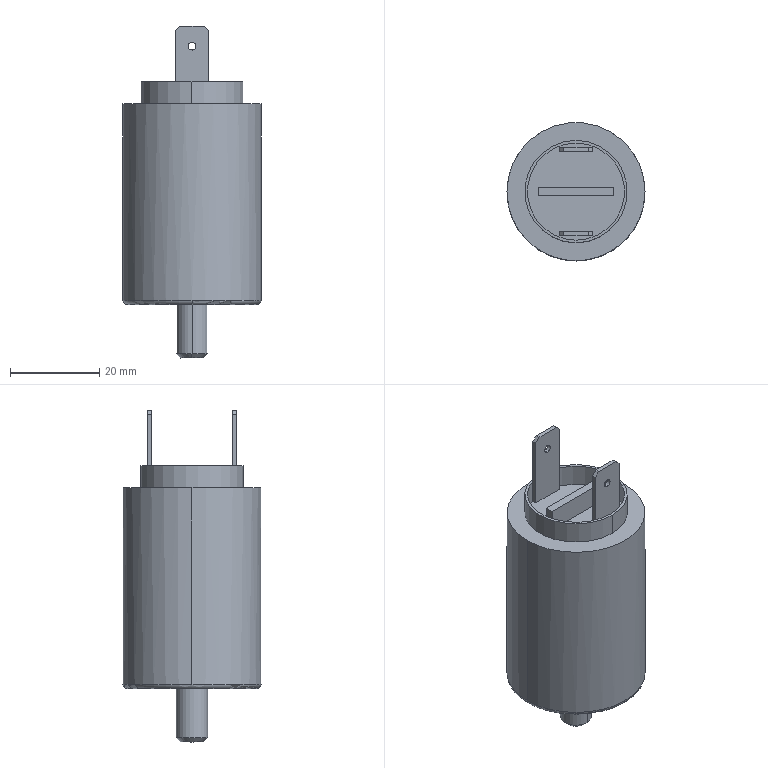Part | STEP file | MSBR-17_1_1_1_1 | 1 solid | 40 faces | box 31 x 31 x 74.5 mm | volume 34990 mm3 | plane 24 | cylinder 12 | torus 2 | cone 2 | commonest cylinder face diameters 1.8 x4 7 x2 21.8 x2 23 x2 31 x2
STEP:
#1=CARTESIAN_POINT('',(0.,0.,0.));
#2=DIRECTION('',(0.,0.,1.));
#3=DIRECTION('',(1.,0.,0.));
#4=AXIS2_PLACEMENT_3D('',#1,#2,#3);
#5=CARTESIAN_POINT('',(10.,61.412,67.3));
#6=VERTEX_POINT('',#5);
#7=CARTESIAN_POINT('',(10.,61.412,62.3));
#8=VERTEX_POINT('',#7);
#9=CARTESIAN_POINT('',(10.,61.412,67.3));
#10=DIRECTION('',(0.,0.,-1.));
#11=VECTOR('',#10,5.);
#12=LINE('',#9,#11);
#13=EDGE_CURVE('',#6,#8,#12,.T.);
#14=ORIENTED_EDGE('',*,*,#13,.F.);
#15=CARTESIAN_POINT('',(10.,83.212,67.3));
#16=VERTEX_POINT('',#15);
#17=CARTESIAN_POINT('',(10.,72.312,67.3));
#18=DIRECTION('',(0.,0.,1.));
#19=DIRECTION('',(0.,1.,0.));
#20=AXIS2_PLACEMENT_3D('',#17,#18,#19);
#21=CIRCLE('',#20,10.9);
#22=EDGE_CURVE('',#16,#6,#21,.T.);
#23=ORIENTED_EDGE('',*,*,#22,.F.);
#24=CARTESIAN_POINT('',(10.,83.212,62.3));
#25=VERTEX_POINT('',#24);
#26=CARTESIAN_POINT('',(10.,83.212,62.3));
#27=DIRECTION('',(0.,0.,1.));
#28=VECTOR('',#27,5.);
#29=LINE('',#26,#28);
#30=EDGE_CURVE('',#25,#16,#29,.T.);
#31=ORIENTED_EDGE('',*,*,#30,.F.);
#32=CARTESIAN_POINT('',(10.,72.312,62.3));
#33=DIRECTION('',(0.,0.,-1.));
#34=DIRECTION('',(0.,-1.,0.));
#35=AXIS2_PLACEMENT_3D('',#32,#33,#34);
#36=CIRCLE('',#35,10.9);
#37=EDGE_CURVE('',#8,#25,#36,.T.);
#38=ORIENTED_EDGE('',*,*,#37,.F.);
#39=EDGE_LOOP('',(#14,#23,#31,#38));
#40=FACE_OUTER_BOUND('',#39,.F.);
#41=CARTESIAN_POINT('',(10.,72.312,62.196));
#42=DIRECTION('',(0.,0.,1.));
#43=DIRECTION('',(0.,1.,0.));
#44=AXIS2_PLACEMENT_3D('',#41,#42,#43);
#45=CYLINDRICAL_SURFACE('',#44,10.9);
#46=ADVANCED_FACE('',(#40),#45,.F.);
#47=CARTESIAN_POINT('',(10.,72.312,67.3));
#48=DIRECTION('',(0.,0.,1.));
#49=DIRECTION('',(0.,-1.,0.));
#50=AXIS2_PLACEMENT_3D('',#47,#48,#49);
#51=CIRCLE('',#50,10.9);
#52=EDGE_CURVE('',#6,#16,#51,.T.);
#53=ORIENTED_EDGE('',*,*,#52,.F.);
#54=ORIENTED_EDGE('',*,*,#13,.T.);
#55=CARTESIAN_POINT('',(10.,72.312,62.3));
#56=DIRECTION('',(0.,0.,-1.));
#57=DIRECTION('',(0.,1.,0.));
#58=AXIS2_PLACEMENT_3D('',#55,#56,#57);
#59=CIRCLE('',#58,10.9);
#60=EDGE_CURVE('',#25,#8,#59,.T.);
#61=ORIENTED_EDGE('',*,*,#60,.F.);
#62=ORIENTED_EDGE('',*,*,#30,.T.);
#63=EDGE_LOOP('',(#53,#54,#61,#62));
#64=FACE_OUTER_BOUND('',#63,.F.);
#65=CARTESIAN_POINT('',(10.,72.312,62.196));
#66=DIRECTION('',(0.,0.,1.));
#67=DIRECTION('',(0.,-1.,0.));
#68=AXIS2_PLACEMENT_3D('',#65,#66,#67);
#69=CYLINDRICAL_SURFACE('',#68,10.9);
#70=ADVANCED_FACE('',(#64),#69,.F.);
#71=CARTESIAN_POINT('',(10.,83.812,67.3));
#72=VERTEX_POINT('',#71);
#73=CARTESIAN_POINT('',(10.,60.812,67.3));
#74=VERTEX_POINT('',#73);
#75=CARTESIAN_POINT('',(10.,72.312,67.3));
#76=DIRECTION('',(0.,0.,-1.));
#77=DIRECTION('',(0.,1.,0.));
#78=AXIS2_PLACEMENT_3D('',#75,#76,#77);
#79=CIRCLE('',#78,11.5);
#80=EDGE_CURVE('',#72,#74,#79,.T.);
#81=ORIENTED_EDGE('',*,*,#80,.T.);
#82=CARTESIAN_POINT('',(10.,72.312,67.3));
#83=DIRECTION('',(0.,0.,-1.));
#84=DIRECTION('',(0.,-1.,0.));
#85=AXIS2_PLACEMENT_3D('',#82,#83,#84);
#86=CIRCLE('',#85,11.5);
#87=EDGE_CURVE('',#74,#72,#86,.T.);
#88=ORIENTED_EDGE('',*,*,#87,.T.);
#89=EDGE_LOOP('',(#81,#88));
#90=FACE_OUTER_BOUND('',#89,.F.);
#91=ORIENTED_EDGE('',*,*,#22,.T.);
#92=ORIENTED_EDGE('',*,*,#52,.T.);
#93=EDGE_LOOP('',(#91,#92));
#94=FACE_BOUND('',#93,.F.);
#95=CARTESIAN_POINT('',(10.,72.312,67.3));
#96=DIRECTION('',(0.,0.,1.));
#97=DIRECTION('',(0.,1.,0.));
#98=AXIS2_PLACEMENT_3D('',#95,#96,#97);
#99=PLANE('',#98);
#100=ADVANCED_FACE('',(#90,#94),#99,.T.);
#101=CARTESIAN_POINT('',(10.,60.812,62.3));
#102=VERTEX_POINT('',#101);
#103=CARTESIAN_POINT('',(10.,83.812,62.3));
#104=VERTEX_POINT('',#103);
#105=CARTESIAN_POINT('',(10.,72.312,62.3));
#106=DIRECTION('',(0.,0.,1.));
#107=DIRECTION('',(0.,-1.,0.));
#108=AXIS2_PLACEMENT_3D('',#105,#106,#107);
#109=CIRCLE('',#108,11.5);
#110=EDGE_CURVE('',#102,#104,#109,.T.);
#111=ORIENTED_EDGE('',*,*,#110,.F.);
#112=CARTESIAN_POINT('',(10.,60.812,67.3));
#113=DIRECTION('',(0.,0.,-1.));
#114=VECTOR('',#113,5.);
#115=LINE('',#112,#114);
#116=EDGE_CURVE('',#74,#102,#115,.T.);
#117=ORIENTED_EDGE('',*,*,#116,.F.);
#118=ORIENTED_EDGE('',*,*,#80,.F.);
#119=CARTESIAN_POINT('',(10.,83.812,62.3));
#120=DIRECTION('',(0.,0.,1.));
#121=VECTOR('',#120,5.);
#122=LINE('',#119,#121);
#123=EDGE_CURVE('',#104,#72,#122,.T.);
#124=ORIENTED_EDGE('',*,*,#123,.F.);
#125=EDGE_LOOP('',(#111,#117,#118,#124));
#126=FACE_OUTER_BOUND('',#125,.F.);
#127=CARTESIAN_POINT('',(10.,72.312,62.196));
#128=DIRECTION('',(0.,0.,1.));
#129=DIRECTION('',(0.,-1.,0.));
#130=AXIS2_PLACEMENT_3D('',#127,#128,#129);
#131=CYLINDRICAL_SURFACE('',#130,11.5);
#132=ADVANCED_FACE('',(#126),#131,.T.);
#133=CARTESIAN_POINT('',(25.5,72.312,62.3));
#134=VERTEX_POINT('',#133);
#135=CARTESIAN_POINT('',(-5.5,72.312,62.3));
#136=VERTEX_POINT('',#135);
#137=CARTESIAN_POINT('',(10.,72.312,62.3));
#138=DIRECTION('',(0.,0.,-1.));
#139=DIRECTION('',(1.,0.,0.));
#140=AXIS2_PLACEMENT_3D('',#137,#138,#139);
#141=CIRCLE('',#140,15.5);
#142=EDGE_CURVE('',#134,#136,#141,.T.);
#143=ORIENTED_EDGE('',*,*,#142,.T.);
#144=CARTESIAN_POINT('',(10.,72.312,62.3));
#145=DIRECTION('',(0.,0.,-1.));
#146=DIRECTION('',(-1.,0.,0.));
#147=AXIS2_PLACEMENT_3D('',#144,#145,#146);
#148=CIRCLE('',#147,15.5);
#149=EDGE_CURVE('',#136,#134,#148,.T.);
#150=ORIENTED_EDGE('',*,*,#149,.T.);
#151=EDGE_LOOP('',(#143,#150));
#152=FACE_OUTER_BOUND('',#151,.F.);
#153=ORIENTED_EDGE('',*,*,#110,.T.);
#154=CARTESIAN_POINT('',(10.,72.312,62.3));
#155=DIRECTION('',(0.,0.,1.));
#156=DIRECTION('',(0.,1.,0.));
#157=AXIS2_PLACEMENT_3D('',#154,#155,#156);
#158=CIRCLE('',#157,11.5);
#159=EDGE_CURVE('',#104,#102,#158,.T.);
#160=ORIENTED_EDGE('',*,*,#159,.T.);
#161=EDGE_LOOP('',(#153,#160));
#162=FACE_BOUND('',#161,.F.);
#163=CARTESIAN_POINT('',(10.,72.312,62.3));
#164=DIRECTION('',(0.,0.,1.));
#165=DIRECTION('',(0.,1.,0.));
#166=AXIS2_PLACEMENT_3D('',#163,#164,#165);
#167=PLANE('',#166);
#168=ADVANCED_FACE('',(#152,#162),#167,.T.);
#169=CARTESIAN_POINT('',(10.,56.812,18.3));
#170=VERTEX_POINT('',#169);
#171=CARTESIAN_POINT('',(25.5,72.312,18.3));
#172=VERTEX_POINT('',#171);
#173=CARTESIAN_POINT('',(10.,72.312,18.3));
#174=DIRECTION('',(0.,0.,1.));
#175=DIRECTION('',(0.,-1.,0.));
#176=AXIS2_PLACEMENT_3D('',#173,#174,#175);
#177=CIRCLE('',#176,15.5);
#178=EDGE_CURVE('',#170,#172,#177,.T.);
#179=ORIENTED_EDGE('',*,*,#178,.F.);
#180=CARTESIAN_POINT('',(-5.5,72.312,18.3));
#181=VERTEX_POINT('',#180);
#182=CARTESIAN_POINT('',(10.,72.312,18.3));
#183=DIRECTION('',(0.,0.,1.));
#184=DIRECTION('',(-1.,0.,0.));
#185=AXIS2_PLACEMENT_3D('',#182,#183,#184);
#186=CIRCLE('',#185,15.5);
#187=EDGE_CURVE('',#181,#170,#186,.T.);
#188=ORIENTED_EDGE('',*,*,#187,.F.);
#189=CARTESIAN_POINT('',(-5.5,72.312,62.3));
#190=DIRECTION('',(0.,0.,-1.));
#191=VECTOR('',#190,44.);
#192=LINE('',#189,#191);
#193=EDGE_CURVE('',#136,#181,#192,.T.);
#194=ORIENTED_EDGE('',*,*,#193,.F.);
#195=ORIENTED_EDGE('',*,*,#142,.F.);
#196=CARTESIAN_POINT('',(25.5,72.312,18.3));
#197=DIRECTION('',(0.,0.,1.));
#198=VECTOR('',#197,44.);
#199=LINE('',#196,#198);
#200=EDGE_CURVE('',#172,#134,#199,.T.);
#201=ORIENTED_EDGE('',*,*,#200,.F.);
#202=EDGE_LOOP('',(#179,#188,#194,#195,#201));
#203=FACE_OUTER_BOUND('',#202,.F.);
#204=CARTESIAN_POINT('',(10.,72.312,17.42));
#205=DIRECTION('',(0.,0.,1.));
#206=DIRECTION('',(-1.,0.,0.));
#207=AXIS2_PLACEMENT_3D('',#204,#205,#206);
#208=CYLINDRICAL_SURFACE('',#207,15.5);
#209=ADVANCED_FACE('',(#203),#208,.T.);
#210=CARTESIAN_POINT('',(10.,57.812,17.3));
#211=VERTEX_POINT('',#210);
#212=CARTESIAN_POINT('',(10.,86.812,17.3));
#213=VERTEX_POINT('',#212);
#214=CARTESIAN_POINT('',(10.,72.312,17.3));
#215=DIRECTION('',(0.,0.,1.));
#216=DIRECTION('',(0.,-1.,0.));
#217=AXIS2_PLACEMENT_3D('',#214,#215,#216);
#218=CIRCLE('',#217,14.5);
#219=EDGE_CURVE('',#211,#213,#218,.T.);
#220=ORIENTED_EDGE('',*,*,#219,.F.);
#221=CARTESIAN_POINT('',(10.,57.812,18.3));
#222=DIRECTION('',(1.,0.,0.));
#223=DIRECTION('',(0.,-1.,0.));
#224=AXIS2_PLACEMENT_3D('',#221,#222,#223);
#225=CIRCLE('',#224,1.);
#226=EDGE_CURVE('',#170,#211,#225,.T.);
#227=ORIENTED_EDGE('',*,*,#226,.F.);
#228=ORIENTED_EDGE('',*,*,#178,.T.);
#229=CARTESIAN_POINT('',(10.,87.812,18.3));
#230=VERTEX_POINT('',#229);
#231=CARTESIAN_POINT('',(10.,72.312,18.3));
#232=DIRECTION('',(0.,0.,1.));
#233=DIRECTION('',(1.,0.,0.));
#234=AXIS2_PLACEMENT_3D('',#231,#232,#233);
#235=CIRCLE('',#234,15.5);
#236=EDGE_CURVE('',#172,#230,#235,.T.);
#237=ORIENTED_EDGE('',*,*,#236,.T.);
#238=CARTESIAN_POINT('',(10.,86.812,18.3));
#239=DIRECTION('',(1.,0.,0.));
#240=DIRECTION('',(0.,0.,-1.));
#241=AXIS2_PLACEMENT_3D('',#238,#239,#240);
#242=CIRCLE('',#241,1.);
#243=EDGE_CURVE('',#213,#230,#242,.T.);
#244=ORIENTED_EDGE('',*,*,#243,.F.);
#245=EDGE_LOOP('',(#220,#227,#228,#237,#244));
#246=FACE_OUTER_BOUND('',#245,.F.);
#247=CARTESIAN_POINT('',(10.,72.312,18.3));
#248=DIRECTION('',(0.,0.,-1.));
#249=DIRECTION('',(0.,-1.,0.));
#250=AXIS2_PLACEMENT_3D('',#247,#248,#249);
#251=TOROIDAL_SURFACE('',#250,14.5,1.);
#252=ADVANCED_FACE('',(#246),#251,.T.);
#253=ORIENTED_EDGE('',*,*,#219,.T.);
#254=CARTESIAN_POINT('',(10.,72.312,17.3));
#255=DIRECTION('',(0.,0.,1.));
#256=DIRECTION('',(0.,1.,0.));
#257=AXIS2_PLACEMENT_3D('',#254,#255,#256);
#258=CIRCLE('',#257,14.5);
#259=EDGE_CURVE('',#213,#211,#258,.T.);
#260=ORIENTED_EDGE('',*,*,#259,.T.);
#261=EDGE_LOOP('',(#253,#260));
#262=FACE_OUTER_BOUND('',#261,.F.);
#263=CARTESIAN_POINT('',(10.,75.812,17.3));
#264=VERTEX_POINT('',#263);
#265=CARTESIAN_POINT('',(10.,68.812,17.3));
#266=VERTEX_POINT('',#265);
#267=CARTESIAN_POINT('',(10.,72.312,17.3));
#268=DIRECTION('',(0.,0.,-1.));
#269=DIRECTION('',(0.,1.,0.));
#270=AXIS2_PLACEMENT_3D('',#267,#268,#269);
#271=CIRCLE('',#270,3.5);
#272=EDGE_CURVE('',#264,#266,#271,.T.);
#273=ORIENTED_EDGE('',*,*,#272,.T.);
#274=CARTESIAN_POINT('',(10.,72.312,17.3));
#275=DIRECTION('',(0.,0.,-1.));
#276=DIRECTION('',(0.,-1.,0.));
#277=AXIS2_PLACEMENT_3D('',#274,#275,#276);
#278=CIRCLE('',#277,3.5);
#279=EDGE_CURVE('',#266,#264,#278,.T.);
#280=ORIENTED_EDGE('',*,*,#279,.T.);
#281=EDGE_LOOP('',(#273,#280));
#282=FACE_BOUND('',#281,.F.);
#283=CARTESIAN_POINT('',(10.,72.312,17.3));
#284=DIRECTION('',(0.,0.,1.));
#285=DIRECTION('',(0.,1.,0.));
#286=AXIS2_PLACEMENT_3D('',#283,#284,#285);
#287=PLANE('',#286);
#288=ADVANCED_FACE('',(#262,#282),#287,.F.);
#289=ORIENTED_EDGE('',*,*,#243,.T.);
#290=CARTESIAN_POINT('',(10.,72.312,18.3));
#291=DIRECTION('',(0.,0.,1.));
#292=DIRECTION('',(0.,1.,0.));
#293=AXIS2_PLACEMENT_3D('',#290,#291,#292);
#294=CIRCLE('',#293,15.5);
#295=EDGE_CURVE('',#230,#181,#294,.T.);
#296=ORIENTED_EDGE('',*,*,#295,.T.);
#297=ORIENTED_EDGE('',*,*,#187,.T.);
#298=ORIENTED_EDGE('',*,*,#226,.T.);
#299=ORIENTED_EDGE('',*,*,#259,.F.);
#300=EDGE_LOOP('',(#289,#296,#297,#298,#299));
#301=FACE_OUTER_BOUND('',#300,.F.);
#302=CARTESIAN_POINT('',(10.,72.312,18.3));
#303=DIRECTION('',(0.,0.,-1.));
#304=DIRECTION('',(0.,1.,0.));
#305=AXIS2_PLACEMENT_3D('',#302,#303,#304);
#306=TOROIDAL_SURFACE('',#305,14.5,1.);
#307=ADVANCED_FACE('',(#301),#306,.T.);
#308=ORIENTED_EDGE('',*,*,#200,.T.);
#309=ORIENTED_EDGE('',*,*,#149,.F.);
#310=ORIENTED_EDGE('',*,*,#193,.T.);
#311=ORIENTED_EDGE('',*,*,#295,.F.);
#312=ORIENTED_EDGE('',*,*,#236,.F.);
#313=EDGE_LOOP('',(#308,#309,#310,#311,#312));
#314=FACE_OUTER_BOUND('',#313,.F.);
#315=CARTESIAN_POINT('',(10.,72.312,17.42));
#316=DIRECTION('',(0.,0.,1.));
#317=DIRECTION('',(1.,0.,0.));
#318=AXIS2_PLACEMENT_3D('',#315,#316,#317);
#319=CYLINDRICAL_SURFACE('',#318,15.5);
#320=ADVANCED_FACE('',(#314),#319,.T.);
#321=CARTESIAN_POINT('',(10.,68.812,6.3));
#322=VERTEX_POINT('',#321);
#323=CARTESIAN_POINT('',(10.,75.812,6.3));
#324=VERTEX_POINT('',#323);
#325=CARTESIAN_POINT('',(10.,72.312,6.3));
#326=DIRECTION('',(0.,0.,1.));
#327=DIRECTION('',(0.,-1.,0.));
#328=AXIS2_PLACEMENT_3D('',#325,#326,#327);
#329=CIRCLE('',#328,3.5);
#330=EDGE_CURVE('',#322,#324,#329,.T.);
#331=ORIENTED_EDGE('',*,*,#330,.F.);
#332=CARTESIAN_POINT('',(10.,68.812,17.3));
#333=DIRECTION('',(0.,-0.000000002,-1.));
#334=VECTOR('',#333,11.);
#335=LINE('',#332,#334);
#336=EDGE_CURVE('',#266,#322,#335,.T.);
#337=ORIENTED_EDGE('',*,*,#336,.F.);
#338=ORIENTED_EDGE('',*,*,#272,.F.);
#339=CARTESIAN_POINT('',(10.,75.812,6.3));
#340=DIRECTION('',(0.,-0.000000002,1.));
#341=VECTOR('',#340,11.);
#342=LINE('',#339,#341);
#343=EDGE_CURVE('',#324,#264,#342,.T.);
#344=ORIENTED_EDGE('',*,*,#343,.F.);
#345=EDGE_LOOP('',(#331,#337,#338,#344));
#346=FACE_OUTER_BOUND('',#345,.F.);
#347=CARTESIAN_POINT('',(10.,72.312,6.08));
#348=DIRECTION('',(0.,0.,1.));
#349=DIRECTION('',(0.,-1.,0.));
#350=AXIS2_PLACEMENT_3D('',#347,#348,#349);
#351=CYLINDRICAL_SURFACE('',#350,3.5);
#352=ADVANCED_FACE('',(#346),#351,.T.);
#353=ORIENTED_EDGE('',*,*,#330,.T.);
#354=CARTESIAN_POINT('',(10.,74.812,5.3));
#355=VERTEX_POINT('',#354);
#356=CARTESIAN_POINT('',(10.,74.812,5.3));
#357=DIRECTION('',(-0.000000004,0.7071,0.7071));
#358=VECTOR('',#357,1.414);
#359=LINE('',#356,#358);
#360=EDGE_CURVE('',#355,#324,#359,.T.);
#361=ORIENTED_EDGE('',*,*,#360,.F.);
#362=CARTESIAN_POINT('',(10.,69.812,5.3));
#363=VERTEX_POINT('',#362);
#364=CARTESIAN_POINT('',(10.,72.312,5.3));
#365=DIRECTION('',(0.,0.,1.));
#366=DIRECTION('',(0.,-1.,0.));
#367=AXIS2_PLACEMENT_3D('',#364,#365,#366);
#368=CIRCLE('',#367,2.5);
#369=EDGE_CURVE('',#363,#355,#368,.T.);
#370=ORIENTED_EDGE('',*,*,#369,.F.);
#371=CARTESIAN_POINT('',(10.,68.812,6.3));
#372=DIRECTION('',(0.,0.7071,-0.7071));
#373=VECTOR('',#372,1.414);
#374=LINE('',#371,#373);
#375=EDGE_CURVE('',#322,#363,#374,.T.);
#376=ORIENTED_EDGE('',*,*,#375,.F.);
#377=EDGE_LOOP('',(#353,#361,#370,#376));
#378=FACE_OUTER_BOUND('',#377,.F.);
#379=CARTESIAN_POINT('',(10.,72.312,5.8));
#380=DIRECTION('',(0.,0.,1.));
#381=DIRECTION('',(0.,1.,0.));
#382=AXIS2_PLACEMENT_3D('',#379,#380,#381);
#383=CONICAL_SURFACE('',#382,3.,45.);
#384=ADVANCED_FACE('',(#378),#383,.T.);
#385=ORIENTED_EDGE('',*,*,#375,.T.);
#386=CARTESIAN_POINT('',(10.,72.312,5.3));
#387=DIRECTION('',(-0.000000001,0.,1.));
#388=DIRECTION('',(0.000000006,1.,0.));
#389=AXIS2_PLACEMENT_3D('',#386,#387,#388);
#390=CIRCLE('',#389,2.5);
#391=EDGE_CURVE('',#355,#363,#390,.T.);
#392=ORIENTED_EDGE('',*,*,#391,.F.);
#393=ORIENTED_EDGE('',*,*,#360,.T.);
#394=CARTESIAN_POINT('',(10.,72.312,6.3));
#395=DIRECTION('',(-0.000000001,0.,1.));
#396=DIRECTION('',(0.,1.,0.));
#397=AXIS2_PLACEMENT_3D('',#394,#395,#396);
#398=CIRCLE('',#397,3.5);
#399=EDGE_CURVE('',#324,#322,#398,.T.);
#400=ORIENTED_EDGE('',*,*,#399,.T.);
#401=EDGE_LOOP('',(#385,#392,#393,#400));
#402=FACE_OUTER_BOUND('',#401,.F.);
#403=CARTESIAN_POINT('',(10.,72.312,5.8));
#404=DIRECTION('',(-0.000000001,0.,1.));
#405=DIRECTION('',(0.,-1.,0.));
#406=AXIS2_PLACEMENT_3D('',#403,#404,#405);
#407=CONICAL_SURFACE('',#406,3.,45.);
#408=ADVANCED_FACE('',(#402),#407,.T.);
#409=ORIENTED_EDGE('',*,*,#391,.T.);
#410=ORIENTED_EDGE('',*,*,#369,.T.);
#411=EDGE_LOOP('',(#409,#410));
#412=FACE_OUTER_BOUND('',#411,.F.);
#413=CARTESIAN_POINT('',(10.,72.312,5.3));
#414=DIRECTION('',(0.,0.,1.));
#415=DIRECTION('',(0.,1.,0.));
#416=AXIS2_PLACEMENT_3D('',#413,#414,#415);
#417=PLANE('',#416);
#418=ADVANCED_FACE('',(#412),#417,.F.);
#419=ORIENTED_EDGE('',*,*,#343,.T.);
#420=ORIENTED_EDGE('',*,*,#279,.F.);
#421=ORIENTED_EDGE('',*,*,#336,.T.);
#422=ORIENTED_EDGE('',*,*,#399,.F.);
#423=EDGE_LOOP('',(#419,#420,#421,#422));
#424=FACE_OUTER_BOUND('',#423,.F.);
#425=CARTESIAN_POINT('',(10.,72.312,6.08));
#426=DIRECTION('',(0.,0.,1.));
#427=DIRECTION('',(0.,1.,0.));
#428=AXIS2_PLACEMENT_3D('',#425,#426,#427);
#429=CYLINDRICAL_SURFACE('',#428,3.5);
#430=ADVANCED_FACE('',(#424),#429,.T.);
#431=ORIENTED_EDGE('',*,*,#123,.T.);
#432=ORIENTED_EDGE('',*,*,#87,.F.);
#433=ORIENTED_EDGE('',*,*,#116,.T.);
#434=ORIENTED_EDGE('',*,*,#159,.F.);
#435=EDGE_LOOP('',(#431,#432,#433,#434));
#436=FACE_OUTER_BOUND('',#435,.F.);
#437=CARTESIAN_POINT('',(10.,72.312,62.196));
#438=DIRECTION('',(0.,0.,1.));
#439=DIRECTION('',(0.,1.,0.));
#440=AXIS2_PLACEMENT_3D('',#437,#438,#439);
#441=CYLINDRICAL_SURFACE('',#440,11.5);
#442=ADVANCED_FACE('',(#436),#441,.T.);
#443=ORIENTED_EDGE('',*,*,#60,.T.);
#444=ORIENTED_EDGE('',*,*,#37,.T.);
#445=EDGE_LOOP('',(#443,#444));
#446=FACE_OUTER_BOUND('',#445,.F.);
#447=CARTESIAN_POINT('',(1.5,71.412,62.3));
#448=VERTEX_POINT('',#447);
#449=CARTESIAN_POINT('',(1.5,73.212,62.3));
#450=VERTEX_POINT('',#449);
#451=CARTESIAN_POINT('',(1.5,71.412,62.3));
#452=DIRECTION('',(0.,1.,0.));
#453=VECTOR('',#452,1.8);
#454=LINE('',#451,#453);
#455=EDGE_CURVE('',#448,#450,#454,.T.);
#456=ORIENTED_EDGE('',*,*,#455,.F.);
#457=CARTESIAN_POINT('',(18.5,71.412,62.3));
#458=VERTEX_POINT('',#457);
#459=CARTESIAN_POINT('',(18.5,71.412,62.3));
#460=DIRECTION('',(-1.,0.,0.));
#461=VECTOR('',#460,17.);
#462=LINE('',#459,#461);
#463=EDGE_CURVE('',#458,#448,#462,.T.);
#464=ORIENTED_EDGE('',*,*,#463,.F.);
#465=CARTESIAN_POINT('',(18.5,73.212,62.3));
#466=VERTEX_POINT('',#465);
#467=CARTESIAN_POINT('',(18.5,73.212,62.3));
#468=DIRECTION('',(0.,-1.,0.));
#469=VECTOR('',#468,1.8);
#470=LINE('',#467,#469);
#471=EDGE_CURVE('',#466,#458,#470,.T.);
#472=ORIENTED_EDGE('',*,*,#471,.F.);
#473=CARTESIAN_POINT('',(1.5,73.212,62.3));
#474=DIRECTION('',(1.,0.,0.));
#475=VECTOR('',#474,17.);
#476=LINE('',#473,#475);
#477=EDGE_CURVE('',#450,#466,#476,.T.);
#478=ORIENTED_EDGE('',*,*,#477,.F.);
#479=EDGE_LOOP('',(#456,#464,#472,#478));
#480=FACE_BOUND('',#479,.F.);
#481=CARTESIAN_POINT('',(13.75,82.212,62.3));
#482=VERTEX_POINT('',#481);
#483=CARTESIAN_POINT('',(13.75,81.312,62.3));
#484=VERTEX_POINT('',#483);
#485=CARTESIAN_POINT('',(13.75,82.212,62.3));
#486=DIRECTION('',(0.,-1.,0.));
#487=VECTOR('',#486,0.9);
#488=LINE('',#485,#487);
#489=EDGE_CURVE('',#482,#484,#488,.T.);
#490=ORIENTED_EDGE('',*,*,#489,.F.);
#491=CARTESIAN_POINT('',(6.25,82.212,62.3));
#492=VERTEX_POINT('',#491);
#493=CARTESIAN_POINT('',(6.25,82.212,62.3));
#494=DIRECTION('',(1.,0.,0.));
#495=VECTOR('',#494,7.5);
#496=LINE('',#493,#495);
#497=EDGE_CURVE('',#492,#482,#496,.T.);
#498=ORIENTED_EDGE('',*,*,#497,.F.);
#499=CARTESIAN_POINT('',(6.25,81.312,62.3));
#500=VERTEX_POINT('',#499);
#501=CARTESIAN_POINT('',(6.25,81.312,62.3));
#502=DIRECTION('',(0.,1.,0.));
#503=VECTOR('',#502,0.9);
#504=LINE('',#501,#503);
#505=EDGE_CURVE('',#500,#492,#504,.T.);
#506=ORIENTED_EDGE('',*,*,#505,.F.);
#507=CARTESIAN_POINT('',(13.75,81.312,62.3));
#508=DIRECTION('',(-1.,0.,0.));
#509=VECTOR('',#508,7.5);
#510=LINE('',#507,#509);
#511=EDGE_CURVE('',#484,#500,#510,.T.);
#512=ORIENTED_EDGE('',*,*,#511,.F.);
#513=EDGE_LOOP('',(#490,#498,#506,#512));
#514=FACE_BOUND('',#513,.F.);
#515=CARTESIAN_POINT('',(13.75,63.312,62.3));
#516=VERTEX_POINT('',#515);
#517=CARTESIAN_POINT('',(13.75,62.412,62.3));
#518=VERTEX_POINT('',#517);
#519=CARTESIAN_POINT('',(13.75,63.312,62.3));
#520=DIRECTION('',(0.,-1.,0.));
#521=VECTOR('',#520,0.9);
#522=LINE('',#519,#521);
#523=EDGE_CURVE('',#516,#518,#522,.T.);
#524=ORIENTED_EDGE('',*,*,#523,.F.);
#525=CARTESIAN_POINT('',(6.25,63.312,62.3));
#526=VERTEX_POINT('',#525);
#527=CARTESIAN_POINT('',(6.25,63.312,62.3));
#528=DIRECTION('',(1.,0.,0.));
#529=VECTOR('',#528,7.5);
#530=LINE('',#527,#529);
#531=EDGE_CURVE('',#526,#516,#530,.T.);
#532=ORIENTED_EDGE('',*,*,#531,.F.);
#533=CARTESIAN_POINT('',(6.25,62.412,62.3));
#534=VERTEX_POINT('',#533);
#535=CARTESIAN_POINT('',(6.25,62.412,62.3));
#536=DIRECTION('',(0.,1.,0.));
#537=VECTOR('',#536,0.9);
#538=LINE('',#535,#537);
#539=EDGE_CURVE('',#534,#526,#538,.T.);
#540=ORIENTED_EDGE('',*,*,#539,.F.);
#541=CARTESIAN_POINT('',(13.75,62.412,62.3));
#542=DIRECTION('',(-1.,0.,0.));
#543=VECTOR('',#542,7.5);
#544=LINE('',#541,#543);
#545=EDGE_CURVE('',#518,#534,#544,.T.);
#546=ORIENTED_EDGE('',*,*,#545,.F.);
#547=EDGE_LOOP('',(#524,#532,#540,#546));
#548=FACE_BOUND('',#547,.F.);
#549=CARTESIAN_POINT('',(10.,72.312,62.3));
#550=DIRECTION('',(0.,0.,1.));
#551=DIRECTION('',(0.,1.,0.));
#552=AXIS2_PLACEMENT_3D('',#549,#550,#551);
#553=PLANE('',#552);
#554=ADVANCED_FACE('',(#446,#480,#514,#548),#553,.T.);
#555=ORIENTED_EDGE('',*,*,#455,.T.);
#556=CARTESIAN_POINT('',(1.5,73.212,67.3));
#557=VERTEX_POINT('',#556);
#558=CARTESIAN_POINT('',(1.5,73.212,67.3));
#559=DIRECTION('',(0.,0.,-1.));
#560=VECTOR('',#559,5.);
#561=LINE('',#558,#560);
#562=EDGE_CURVE('',#557,#450,#561,.T.);
#563=ORIENTED_EDGE('',*,*,#562,.F.);
#564=CARTESIAN_POINT('',(1.5,71.412,67.3));
#565=VERTEX_POINT('',#564);
#566=CARTESIAN_POINT('',(1.5,71.412,67.3));
#567=DIRECTION('',(0.,1.,0.));
#568=VECTOR('',#567,1.8);
#569=LINE('',#566,#568);
#570=EDGE_CURVE('',#565,#557,#569,.T.);
#571=ORIENTED_EDGE('',*,*,#570,.F.);
#572=CARTESIAN_POINT('',(1.5,71.412,62.3));
#573=DIRECTION('',(0.,0.,1.));
#574=VECTOR('',#573,5.);
#575=LINE('',#572,#574);
#576=EDGE_CURVE('',#448,#565,#575,.T.);
#577=ORIENTED_EDGE('',*,*,#576,.F.);
#578=EDGE_LOOP('',(#555,#563,#571,#577));
#579=FACE_OUTER_BOUND('',#578,.F.);
#580=CARTESIAN_POINT('',(1.5,72.312,64.8));
#581=DIRECTION('',(1.,0.,0.));
#582=DIRECTION('',(0.,1.,0.));
#583=AXIS2_PLACEMENT_3D('',#580,#581,#582);
#584=PLANE('',#583);
#585=ADVANCED_FACE('',(#579),#584,.F.);
#586=ORIENTED_EDGE('',*,*,#477,.T.);
#587=CARTESIAN_POINT('',(18.5,73.212,67.3));
#588=VERTEX_POINT('',#587);
#589=CARTESIAN_POINT('',(18.5,73.212,67.3));
#590=DIRECTION('',(0.,0.,-1.));
#591=VECTOR('',#590,5.);
#592=LINE('',#589,#591);
#593=EDGE_CURVE('',#588,#466,#592,.T.);
#594=ORIENTED_EDGE('',*,*,#593,.F.);
#595=CARTESIAN_POINT('',(1.5,73.212,67.3));
#596=DIRECTION('',(1.,0.,0.));
#597=VECTOR('',#596,17.);
#598=LINE('',#595,#597);
#599=EDGE_CURVE('',#557,#588,#598,.T.);
#600=ORIENTED_EDGE('',*,*,#599,.F.);
#601=ORIENTED_EDGE('',*,*,#562,.T.);
#602=EDGE_LOOP('',(#586,#594,#600,#601));
#603=FACE_OUTER_BOUND('',#602,.F.);
#604=CARTESIAN_POINT('',(10.,73.212,64.8));
#605=DIRECTION('',(0.,1.,0.));
#606=DIRECTION('',(1.,0.,0.));
#607=AXIS2_PLACEMENT_3D('',#604,#605,#606);
#608=PLANE('',#607);
#609=ADVANCED_FACE('',(#603),#608,.T.);
#610=ORIENTED_EDGE('',*,*,#471,.T.);
#611=CARTESIAN_POINT('',(18.5,71.412,67.3));
#612=VERTEX_POINT('',#611);
#613=CARTESIAN_POINT('',(18.5,71.412,67.3));
#614=DIRECTION('',(0.,0.,-1.));
#615=VECTOR('',#614,5.);
#616=LINE('',#613,#615);
#617=EDGE_CURVE('',#612,#458,#616,.T.);
#618=ORIENTED_EDGE('',*,*,#617,.F.);
#619=CARTESIAN_POINT('',(18.5,73.212,67.3));
#620=DIRECTION('',(0.,-1.,0.));
#621=VECTOR('',#620,1.8);
#622=LINE('',#619,#621);
#623=EDGE_CURVE('',#588,#612,#622,.T.);
#624=ORIENTED_EDGE('',*,*,#623,.F.);
#625=ORIENTED_EDGE('',*,*,#593,.T.);
#626=EDGE_LOOP('',(#610,#618,#624,#625));
#627=FACE_OUTER_BOUND('',#626,.F.);
#628=CARTESIAN_POINT('',(18.5,72.312,64.8));
#629=DIRECTION('',(1.,0.,0.));
#630=DIRECTION('',(0.,-1.,0.));
#631=AXIS2_PLACEMENT_3D('',#628,#629,#630);
#632=PLANE('',#631);
#633=ADVANCED_FACE('',(#627),#632,.T.);
#634=ORIENTED_EDGE('',*,*,#463,.T.);
#635=ORIENTED_EDGE('',*,*,#576,.T.);
#636=CARTESIAN_POINT('',(18.5,71.412,67.3));
#637=DIRECTION('',(-1.,0.,0.));
#638=VECTOR('',#637,17.);
#639=LINE('',#636,#638);
#640=EDGE_CURVE('',#612,#565,#639,.T.);
#641=ORIENTED_EDGE('',*,*,#640,.F.);
#642=ORIENTED_EDGE('',*,*,#617,.T.);
#643=EDGE_LOOP('',(#634,#635,#641,#642));
#644=FACE_OUTER_BOUND('',#643,.F.);
#645=CARTESIAN_POINT('',(10.,71.412,64.8));
#646=DIRECTION('',(0.,1.,0.));
#647=DIRECTION('',(-1.,0.,0.));
#648=AXIS2_PLACEMENT_3D('',#645,#646,#647);
#649=PLANE('',#648);
#650=ADVANCED_FACE('',(#644),#649,.F.);
#651=ORIENTED_EDGE('',*,*,#570,.T.);
#652=ORIENTED_EDGE('',*,*,#599,.T.);
#653=ORIENTED_EDGE('',*,*,#623,.T.);
#654=ORIENTED_EDGE('',*,*,#640,.T.);
#655=EDGE_LOOP('',(#651,#652,#653,#654));
#656=FACE_OUTER_BOUND('',#655,.F.);
#657=CARTESIAN_POINT('',(10.,72.312,67.3));
#658=DIRECTION('',(0.,0.,1.));
#659=DIRECTION('',(0.,1.,0.));
#660=AXIS2_PLACEMENT_3D('',#657,#658,#659);
#661=PLANE('',#660);
#662=ADVANCED_FACE('',(#656),#661,.T.);
#663=CARTESIAN_POINT('',(13.75,82.212,78.8));
#664=VERTEX_POINT('',#663);
#665=CARTESIAN_POINT('',(13.75,82.212,62.3));
#666=DIRECTION('',(0.,0.,1.));
#667=VECTOR('',#666,16.5);
#668=LINE('',#665,#667);
#669=EDGE_CURVE('',#482,#664,#668,.T.);
#670=ORIENTED_EDGE('',*,*,#669,.F.);
#671=ORIENTED_EDGE('',*,*,#489,.T.);
#672=CARTESIAN_POINT('',(13.75,81.312,78.8));
#673=VERTEX_POINT('',#672);
#674=CARTESIAN_POINT('',(13.75,81.312,78.8));
#675=DIRECTION('',(0.,0.,-1.));
#676=VECTOR('',#675,16.5);
#677=LINE('',#674,#676);
#678=EDGE_CURVE('',#673,#484,#677,.T.);
#679=ORIENTED_EDGE('',*,*,#678,.F.);
#680=CARTESIAN_POINT('',(13.75,82.212,78.8));
#681=DIRECTION('',(0.,-1.,0.));
#682=VECTOR('',#681,0.9);
#683=LINE('',#680,#682);
#684=EDGE_CURVE('',#664,#673,#683,.T.);
#685=ORIENTED_EDGE('',*,*,#684,.F.);
#686=EDGE_LOOP('',(#670,#671,#679,#685));
#687=FACE_OUTER_BOUND('',#686,.F.);
#688=CARTESIAN_POINT('',(13.75,81.762,70.55));
#689=DIRECTION('',(1.,0.,0.));
#690=DIRECTION('',(0.,1.,0.));
#691=AXIS2_PLACEMENT_3D('',#688,#689,#690);
#692=PLANE('',#691);
#693=ADVANCED_FACE('',(#687),#692,.T.);
#694=CARTESIAN_POINT('',(6.25,82.212,78.8));
#695=VERTEX_POINT('',#694);
#696=CARTESIAN_POINT('',(6.25,82.212,62.3));
#697=DIRECTION('',(0.,0.,1.));
#698=VECTOR('',#697,16.5);
#699=LINE('',#696,#698);
#700=EDGE_CURVE('',#492,#695,#699,.T.);
#701=ORIENTED_EDGE('',*,*,#700,.F.);
#702=ORIENTED_EDGE('',*,*,#497,.T.);
#703=ORIENTED_EDGE('',*,*,#669,.T.);
#704=CARTESIAN_POINT('',(12.75,82.212,79.8));
#705=VERTEX_POINT('',#704);
#706=CARTESIAN_POINT('',(13.75,82.212,78.8));
#707=DIRECTION('',(-0.7071,0.,0.7071));
#708=VECTOR('',#707,1.414);
#709=LINE('',#706,#708);
#710=EDGE_CURVE('',#664,#705,#709,.T.);
#711=ORIENTED_EDGE('',*,*,#710,.T.);
#712=CARTESIAN_POINT('',(7.25,82.212,79.8));
#713=VERTEX_POINT('',#712);
#714=CARTESIAN_POINT('',(7.25,82.212,79.8));
#715=DIRECTION('',(1.,0.,0.));
#716=VECTOR('',#715,5.5);
#717=LINE('',#714,#716);
#718=EDGE_CURVE('',#713,#705,#717,.T.);
#719=ORIENTED_EDGE('',*,*,#718,.F.);
#720=CARTESIAN_POINT('',(7.25,82.212,79.8));
#721=DIRECTION('',(-0.7071,0.,-0.7071));
#722=VECTOR('',#721,1.414);
#723=LINE('',#720,#722);
#724=EDGE_CURVE('',#713,#695,#723,.T.);
#725=ORIENTED_EDGE('',*,*,#724,.T.);
#726=EDGE_LOOP('',(#701,#702,#703,#711,#719,#725));
#727=FACE_OUTER_BOUND('',#726,.F.);
#728=CARTESIAN_POINT('',(10.,82.212,74.4));
#729=VERTEX_POINT('',#728);
#730=CARTESIAN_POINT('',(10.,82.212,76.2));
#731=VERTEX_POINT('',#730);
#732=CARTESIAN_POINT('',(10.,82.212,75.3));
#733=DIRECTION('',(0.,1.,0.));
#734=DIRECTION('',(0.,0.,-1.));
#735=AXIS2_PLACEMENT_3D('',#732,#733,#734);
#736=CIRCLE('',#735,0.9);
#737=EDGE_CURVE('',#729,#731,#736,.T.);
#738=ORIENTED_EDGE('',*,*,#737,.T.);
#739=CARTESIAN_POINT('',(10.,82.212,75.3));
#740=DIRECTION('',(0.,1.,0.));
#741=DIRECTION('',(0.,0.,1.));
#742=AXIS2_PLACEMENT_3D('',#739,#740,#741);
#743=CIRCLE('',#742,0.9);
#744=EDGE_CURVE('',#731,#729,#743,.T.);
#745=ORIENTED_EDGE('',*,*,#744,.T.);
#746=EDGE_LOOP('',(#738,#745));
#747=FACE_BOUND('',#746,.F.);
#748=CARTESIAN_POINT('',(10.,82.212,71.05));
#749=DIRECTION('',(0.,1.,0.));
#750=DIRECTION('',(-1.,0.,0.));
#751=AXIS2_PLACEMENT_3D('',#748,#749,#750);
#752=PLANE('',#751);
#753=ADVANCED_FACE('',(#727,#747),#752,.T.);
#754=CARTESIAN_POINT('',(6.25,81.312,78.8));
#755=VERTEX_POINT('',#754);
#756=CARTESIAN_POINT('',(6.25,81.312,62.3));
#757=DIRECTION('',(0.,0.,1.));
#758=VECTOR('',#757,16.5);
#759=LINE('',#756,#758);
#760=EDGE_CURVE('',#500,#755,#759,.T.);
#761=ORIENTED_EDGE('',*,*,#760,.F.);
#762=ORIENTED_EDGE('',*,*,#505,.T.);
#763=ORIENTED_EDGE('',*,*,#700,.T.);
#764=CARTESIAN_POINT('',(6.25,81.312,78.8));
#765=DIRECTION('',(0.,1.,0.));
#766=VECTOR('',#765,0.9);
#767=LINE('',#764,#766);
#768=EDGE_CURVE('',#755,#695,#767,.T.);
#769=ORIENTED_EDGE('',*,*,#768,.F.);
#770=EDGE_LOOP('',(#761,#762,#763,#769));
#771=FACE_OUTER_BOUND('',#770,.F.);
#772=CARTESIAN_POINT('',(6.25,81.762,70.55));
#773=DIRECTION('',(1.,0.,0.));
#774=DIRECTION('',(0.,-1.,0.));
#775=AXIS2_PLACEMENT_3D('',#772,#773,#774);
#776=PLANE('',#775);
#777=ADVANCED_FACE('',(#771),#776,.F.);
#778=ORIENTED_EDGE('',*,*,#678,.T.);
#779=ORIENTED_EDGE('',*,*,#511,.T.);
#780=ORIENTED_EDGE('',*,*,#760,.T.);
#781=CARTESIAN_POINT('',(7.25,81.312,79.8));
#782=VERTEX_POINT('',#781);
#783=CARTESIAN_POINT('',(6.25,81.312,78.8));
#784=DIRECTION('',(0.7071,0.,0.7071));
#785=VECTOR('',#784,1.414);
#786=LINE('',#783,#785);
#787=EDGE_CURVE('',#755,#782,#786,.T.);
#788=ORIENTED_EDGE('',*,*,#787,.T.);
#789=CARTESIAN_POINT('',(12.75,81.312,79.8));
#790=VERTEX_POINT('',#789);
#791=CARTESIAN_POINT('',(12.75,81.312,79.8));
#792=DIRECTION('',(-1.,0.,0.));
#793=VECTOR('',#792,5.5);
#794=LINE('',#791,#793);
#795=EDGE_CURVE('',#790,#782,#794,.T.);
#796=ORIENTED_EDGE('',*,*,#795,.F.);
#797=CARTESIAN_POINT('',(12.75,81.312,79.8));
#798=DIRECTION('',(0.7071,0.,-0.7071));
#799=VECTOR('',#798,1.414);
#800=LINE('',#797,#799);
#801=EDGE_CURVE('',#790,#673,#800,.T.);
#802=ORIENTED_EDGE('',*,*,#801,.T.);
#803=EDGE_LOOP('',(#778,#779,#780,#788,#796,#802));
#804=FACE_OUTER_BOUND('',#803,.F.);
#805=CARTESIAN_POINT('',(10.,81.312,74.4));
#806=VERTEX_POINT('',#805);
#807=CARTESIAN_POINT('',(10.,81.312,76.2));
#808=VERTEX_POINT('',#807);
#809=CARTESIAN_POINT('',(10.,81.312,75.3));
#810=DIRECTION('',(0.,-1.,0.));
#811=DIRECTION('',(0.,0.,-1.));
#812=AXIS2_PLACEMENT_3D('',#809,#810,#811);
#813=CIRCLE('',#812,0.9);
#814=EDGE_CURVE('',#806,#808,#813,.T.);
#815=ORIENTED_EDGE('',*,*,#814,.T.);
#816=CARTESIAN_POINT('',(10.,81.312,75.3));
#817=DIRECTION('',(0.,-1.,0.));
#818=DIRECTION('',(0.,0.,1.));
#819=AXIS2_PLACEMENT_3D('',#816,#817,#818);
#820=CIRCLE('',#819,0.9);
#821=EDGE_CURVE('',#808,#806,#820,.T.);
#822=ORIENTED_EDGE('',*,*,#821,.T.);
#823=EDGE_LOOP('',(#815,#822));
#824=FACE_BOUND('',#823,.F.);
#825=CARTESIAN_POINT('',(10.,81.312,71.05));
#826=DIRECTION('',(0.,1.,0.));
#827=DIRECTION('',(1.,0.,0.));
#828=AXIS2_PLACEMENT_3D('',#825,#826,#827);
#829=PLANE('',#828);
#830=ADVANCED_FACE('',(#804,#824),#829,.F.);
#831=ORIENTED_EDGE('',*,*,#787,.F.);
#832=ORIENTED_EDGE('',*,*,#768,.T.);
#833=ORIENTED_EDGE('',*,*,#724,.F.);
#834=CARTESIAN_POINT('',(7.25,81.312,79.8));
#835=DIRECTION('',(0.,1.,0.));
#836=VECTOR('',#835,0.9);
#837=LINE('',#834,#836);
#838=EDGE_CURVE('',#782,#713,#837,.T.);
#839=ORIENTED_EDGE('',*,*,#838,.F.);
#840=EDGE_LOOP('',(#831,#832,#833,#839));
#841=FACE_OUTER_BOUND('',#840,.F.);
#842=CARTESIAN_POINT('',(6.75,81.762,79.3));
#843=DIRECTION('',(0.7071,0.,-0.7071));
#844=DIRECTION('',(-0.7071,0.,-0.7071));
#845=AXIS2_PLACEMENT_3D('',#842,#843,#844);
#846=PLANE('',#845);
#847=ADVANCED_FACE('',(#841),#846,.F.);
#848=CARTESIAN_POINT('',(12.75,81.312,79.8));
#849=DIRECTION('',(0.,1.,0.));
#850=VECTOR('',#849,0.9);
#851=LINE('',#848,#850);
#852=EDGE_CURVE('',#790,#705,#851,.T.);
#853=ORIENTED_EDGE('',*,*,#852,.F.);
#854=ORIENTED_EDGE('',*,*,#795,.T.);
#855=ORIENTED_EDGE('',*,*,#838,.T.);
#856=ORIENTED_EDGE('',*,*,#718,.T.);
#857=EDGE_LOOP('',(#853,#854,#855,#856));
#858=FACE_OUTER_BOUND('',#857,.F.);
#859=CARTESIAN_POINT('',(10.,81.762,79.8));
#860=DIRECTION('',(0.,0.,1.));
#861=DIRECTION('',(0.,1.,0.));
#862=AXIS2_PLACEMENT_3D('',#859,#860,#861);
#863=PLANE('',#862);
#864=ADVANCED_FACE('',(#858),#863,.T.);
#865=ORIENTED_EDGE('',*,*,#710,.F.);
#866=ORIENTED_EDGE('',*,*,#684,.T.);
#867=ORIENTED_EDGE('',*,*,#801,.F.);
#868=ORIENTED_EDGE('',*,*,#852,.T.);
#869=EDGE_LOOP('',(#865,#866,#867,#868));
#870=FACE_OUTER_BOUND('',#869,.F.);
#871=CARTESIAN_POINT('',(13.25,81.762,79.3));
#872=DIRECTION('',(0.7071,0.,0.7071));
#873=DIRECTION('',(0.7071,0.,-0.7071));
#874=AXIS2_PLACEMENT_3D('',#871,#872,#873);
#875=PLANE('',#874);
#876=ADVANCED_FACE('',(#870),#875,.T.);
#877=ORIENTED_EDGE('',*,*,#744,.F.);
#878=CARTESIAN_POINT('',(10.,81.312,76.2));
#879=DIRECTION('',(0.,1.,0.));
#880=VECTOR('',#879,0.9);
#881=LINE('',#878,#880);
#882=EDGE_CURVE('',#808,#731,#881,.T.);
#883=ORIENTED_EDGE('',*,*,#882,.F.);
#884=ORIENTED_EDGE('',*,*,#814,.F.);
#885=CARTESIAN_POINT('',(10.,82.212,74.4));
#886=DIRECTION('',(0.,-1.,0.));
#887=VECTOR('',#886,0.9);
#888=LINE('',#885,#887);
#889=EDGE_CURVE('',#729,#806,#888,.T.);
#890=ORIENTED_EDGE('',*,*,#889,.F.);
#891=EDGE_LOOP('',(#877,#883,#884,#890));
#892=FACE_OUTER_BOUND('',#891,.F.);
#893=CARTESIAN_POINT('',(10.,81.208,75.3));
#894=DIRECTION('',(0.,1.,0.));
#895=DIRECTION('',(0.,0.,1.));
#896=AXIS2_PLACEMENT_3D('',#893,#894,#895);
#897=CYLINDRICAL_SURFACE('',#896,0.9);
#898=ADVANCED_FACE('',(#892),#897,.F.);
#899=ORIENTED_EDGE('',*,*,#882,.T.);
#900=ORIENTED_EDGE('',*,*,#737,.F.);
#901=ORIENTED_EDGE('',*,*,#889,.T.);
#902=ORIENTED_EDGE('',*,*,#821,.F.);
#903=EDGE_LOOP('',(#899,#900,#901,#902));
#904=FACE_OUTER_BOUND('',#903,.F.);
#905=CARTESIAN_POINT('',(10.,81.208,75.3));
#906=DIRECTION('',(0.,1.,0.));
#907=DIRECTION('',(0.,0.,-1.));
#908=AXIS2_PLACEMENT_3D('',#905,#906,#907);
#909=CYLINDRICAL_SURFACE('',#908,0.9);
#910=ADVANCED_FACE('',(#904),#909,.F.);
#911=CARTESIAN_POINT('',(13.75,63.312,78.8));
#912=VERTEX_POINT('',#911);
#913=CARTESIAN_POINT('',(13.75,63.312,62.3));
#914=DIRECTION('',(0.,0.,1.));
#915=VECTOR('',#914,16.5);
#916=LINE('',#913,#915);
#917=EDGE_CURVE('',#516,#912,#916,.T.);
#918=ORIENTED_EDGE('',*,*,#917,.F.);
#919=ORIENTED_EDGE('',*,*,#523,.T.);
#920=CARTESIAN_POINT('',(13.75,62.412,78.8));
#921=VERTEX_POINT('',#920);
#922=CARTESIAN_POINT('',(13.75,62.412,78.8));
#923=DIRECTION('',(0.,0.,-1.));
#924=VECTOR('',#923,16.5);
#925=LINE('',#922,#924);
#926=EDGE_CURVE('',#921,#518,#925,.T.);
#927=ORIENTED_EDGE('',*,*,#926,.F.);
#928=CARTESIAN_POINT('',(13.75,63.312,78.8));
#929=DIRECTION('',(0.,-1.,0.));
#930=VECTOR('',#929,0.9);
#931=LINE('',#928,#930);
#932=EDGE_CURVE('',#912,#921,#931,.T.);
#933=ORIENTED_EDGE('',*,*,#932,.F.);
#934=EDGE_LOOP('',(#918,#919,#927,#933));
#935=FACE_OUTER_BOUND('',#934,.F.);
#936=CARTESIAN_POINT('',(13.75,62.862,70.55));
#937=DIRECTION('',(1.,0.,0.));
#938=DIRECTION('',(0.,1.,0.));
#939=AXIS2_PLACEMENT_3D('',#936,#937,#938);
#940=PLANE('',#939);
#941=ADVANCED_FACE('',(#935),#940,.T.);
#942=CARTESIAN_POINT('',(6.25,63.312,78.8));
#943=VERTEX_POINT('',#942);
#944=CARTESIAN_POINT('',(6.25,63.312,62.3));
#945=DIRECTION('',(0.,0.,1.));
#946=VECTOR('',#945,16.5);
#947=LINE('',#944,#946);
#948=EDGE_CURVE('',#526,#943,#947,.T.);
#949=ORIENTED_EDGE('',*,*,#948,.F.);
#950=ORIENTED_EDGE('',*,*,#531,.T.);
#951=ORIENTED_EDGE('',*,*,#917,.T.);
#952=CARTESIAN_POINT('',(12.75,63.312,79.8));
#953=VERTEX_POINT('',#952);
#954=CARTESIAN_POINT('',(13.75,63.312,78.8));
#955=DIRECTION('',(-0.7071,0.,0.7071));
#956=VECTOR('',#955,1.414);
#957=LINE('',#954,#956);
#958=EDGE_CURVE('',#912,#953,#957,.T.);
#959=ORIENTED_EDGE('',*,*,#958,.T.);
#960=CARTESIAN_POINT('',(7.25,63.312,79.8));
#961=VERTEX_POINT('',#960);
#962=CARTESIAN_POINT('',(7.25,63.312,79.8));
#963=DIRECTION('',(1.,0.,0.));
#964=VECTOR('',#963,5.5);
#965=LINE('',#962,#964);
#966=EDGE_CURVE('',#961,#953,#965,.T.);
#967=ORIENTED_EDGE('',*,*,#966,.F.);
#968=CARTESIAN_POINT('',(7.25,63.312,79.8));
#969=DIRECTION('',(-0.7071,0.,-0.7071));
#970=VECTOR('',#969,1.414);
#971=LINE('',#968,#970);
#972=EDGE_CURVE('',#961,#943,#971,.T.);
#973=ORIENTED_EDGE('',*,*,#972,.T.);
#974=EDGE_LOOP('',(#949,#950,#951,#959,#967,#973));
#975=FACE_OUTER_BOUND('',#974,.F.);
#976=CARTESIAN_POINT('',(10.,63.312,74.4));
#977=VERTEX_POINT('',#976);
#978=CARTESIAN_POINT('',(10.,63.312,76.2));
#979=VERTEX_POINT('',#978);
#980=CARTESIAN_POINT('',(10.,63.312,75.3));
#981=DIRECTION('',(0.,1.,0.));
#982=DIRECTION('',(0.,0.,-1.));
#983=AXIS2_PLACEMENT_3D('',#980,#981,#982);
#984=CIRCLE('',#983,0.9);
#985=EDGE_CURVE('',#977,#979,#984,.T.);
#986=ORIENTED_EDGE('',*,*,#985,.T.);
#987=CARTESIAN_POINT('',(10.,63.312,75.3));
#988=DIRECTION('',(0.,1.,0.));
#989=DIRECTION('',(0.,0.,1.));
#990=AXIS2_PLACEMENT_3D('',#987,#988,#989);
#991=CIRCLE('',#990,0.9);
#992=EDGE_CURVE('',#979,#977,#991,.T.);
#993=ORIENTED_EDGE('',*,*,#992,.T.);
#994=EDGE_LOOP('',(#986,#993));
#995=FACE_BOUND('',#994,.F.);
#996=CARTESIAN_POINT('',(10.,63.312,71.05));
#997=DIRECTION('',(0.,1.,0.));
#998=DIRECTION('',(-1.,0.,0.));
#999=AXIS2_PLACEMENT_3D('',#996,#997,#998);
#1000=PLANE('',#999);
#1001=ADVANCED_FACE('',(#975,#995),#1000,.T.);
#1002=CARTESIAN_POINT('',(6.25,62.412,78.8));
#1003=VERTEX_POINT('',#1002);
#1004=CARTESIAN_POINT('',(6.25,62.412,62.3));
#1005=DIRECTION('',(0.,0.,1.));
#1006=VECTOR('',#1005,16.5);
#1007=LINE('',#1004,#1006);
#1008=EDGE_CURVE('',#534,#1003,#1007,.T.);
#1009=ORIENTED_EDGE('',*,*,#1008,.F.);
#1010=ORIENTED_EDGE('',*,*,#539,.T.);
#1011=ORIENTED_EDGE('',*,*,#948,.T.);
#1012=CARTESIAN_POINT('',(6.25,62.412,78.8));
#1013=DIRECTION('',(0.,1.,0.));
#1014=VECTOR('',#1013,0.9);
#1015=LINE('',#1012,#1014);
#1016=EDGE_CURVE('',#1003,#943,#1015,.T.);
#1017=ORIENTED_EDGE('',*,*,#1016,.F.);
#1018=EDGE_LOOP('',(#1009,#1010,#1011,#1017));
#1019=FACE_OUTER_BOUND('',#1018,.F.);
#1020=CARTESIAN_POINT('',(6.25,62.862,70.55));
#1021=DIRECTION('',(1.,0.,0.));
#1022=DIRECTION('',(0.,-1.,0.));
#1023=AXIS2_PLACEMENT_3D('',#1020,#1021,#1022);
#1024=PLANE('',#1023);
#1025=ADVANCED_FACE('',(#1019),#1024,.F.);
#1026=ORIENTED_EDGE('',*,*,#926,.T.);
#1027=ORIENTED_EDGE('',*,*,#545,.T.);
#1028=ORIENTED_EDGE('',*,*,#1008,.T.);
#1029=CARTESIAN_POINT('',(7.25,62.412,79.8));
#1030=VERTEX_POINT('',#1029);
#1031=CARTESIAN_POINT('',(6.25,62.412,78.8));
#1032=DIRECTION('',(0.7071,0.,0.7071));
#1033=VECTOR('',#1032,1.414);
#1034=LINE('',#1031,#1033);
#1035=EDGE_CURVE('',#1003,#1030,#1034,.T.);
#1036=ORIENTED_EDGE('',*,*,#1035,.T.);
#1037=CARTESIAN_POINT('',(12.75,62.412,79.8));
#1038=VERTEX_POINT('',#1037);
#1039=CARTESIAN_POINT('',(12.75,62.412,79.8));
#1040=DIRECTION('',(-1.,0.,0.));
#1041=VECTOR('',#1040,5.5);
#1042=LINE('',#1039,#1041);
#1043=EDGE_CURVE('',#1038,#1030,#1042,.T.);
#1044=ORIENTED_EDGE('',*,*,#1043,.F.);
#1045=CARTESIAN_POINT('',(12.75,62.412,79.8));
#1046=DIRECTION('',(0.7071,0.,-0.7071));
#1047=VECTOR('',#1046,1.414);
#1048=LINE('',#1045,#1047);
#1049=EDGE_CURVE('',#1038,#921,#1048,.T.);
#1050=ORIENTED_EDGE('',*,*,#1049,.T.);
#1051=EDGE_LOOP('',(#1026,#1027,#1028,#1036,#1044,#1050));
#1052=FACE_OUTER_BOUND('',#1051,.F.);
#1053=CARTESIAN_POINT('',(10.,62.412,74.4));
#1054=VERTEX_POINT('',#1053);
#1055=CARTESIAN_POINT('',(10.,62.412,76.2));
#1056=VERTEX_POINT('',#1055);
#1057=CARTESIAN_POINT('',(10.,62.412,75.3));
#1058=DIRECTION('',(0.,-1.,0.));
#1059=DIRECTION('',(0.,0.,-1.));
#1060=AXIS2_PLACEMENT_3D('',#1057,#1058,#1059);
#1061=CIRCLE('',#1060,0.9);
#1062=EDGE_CURVE('',#1054,#1056,#1061,.T.);
#1063=ORIENTED_EDGE('',*,*,#1062,.T.);
#1064=CARTESIAN_POINT('',(10.,62.412,75.3));
#1065=DIRECTION('',(0.,-1.,0.));
#1066=DIRECTION('',(0.,0.,1.));
#1067=AXIS2_PLACEMENT_3D('',#1064,#1065,#1066);
#1068=CIRCLE('',#1067,0.9);
#1069=EDGE_CURVE('',#1056,#1054,#1068,.T.);
#1070=ORIENTED_EDGE('',*,*,#1069,.T.);
#1071=EDGE_LOOP('',(#1063,#1070));
#1072=FACE_BOUND('',#1071,.F.);
#1073=CARTESIAN_POINT('',(10.,62.412,71.05));
#1074=DIRECTION('',(0.,1.,0.));
#1075=DIRECTION('',(1.,0.,0.));
#1076=AXIS2_PLACEMENT_3D('',#1073,#1074,#1075);
#1077=PLANE('',#1076);
#1078=ADVANCED_FACE('',(#1052,#1072),#1077,.F.);
#1079=ORIENTED_EDGE('',*,*,#1035,.F.);
#1080=ORIENTED_EDGE('',*,*,#1016,.T.);
#1081=ORIENTED_EDGE('',*,*,#972,.F.);
#1082=CARTESIAN_POINT('',(7.25,62.412,79.8));
#1083=DIRECTION('',(0.,1.,0.));
#1084=VECTOR('',#1083,0.9);
#1085=LINE('',#1082,#1084);
#1086=EDGE_CURVE('',#1030,#961,#1085,.T.);
#1087=ORIENTED_EDGE('',*,*,#1086,.F.);
#1088=EDGE_LOOP('',(#1079,#1080,#1081,#1087));
#1089=FACE_OUTER_BOUND('',#1088,.F.);
#1090=CARTESIAN_POINT('',(6.75,62.862,79.3));
#1091=DIRECTION('',(0.7071,0.,-0.7071));
#1092=DIRECTION('',(-0.7071,0.,-0.7071));
#1093=AXIS2_PLACEMENT_3D('',#1090,#1091,#1092);
#1094=PLANE('',#1093);
#1095=ADVANCED_FACE('',(#1089),#1094,.F.);
#1096=CARTESIAN_POINT('',(12.75,62.412,79.8));
#1097=DIRECTION('',(0.,1.,0.));
#1098=VECTOR('',#1097,0.9);
#1099=LINE('',#1096,#1098);
#1100=EDGE_CURVE('',#1038,#953,#1099,.T.);
#1101=ORIENTED_EDGE('',*,*,#1100,.F.);
#1102=ORIENTED_EDGE('',*,*,#1043,.T.);
#1103=ORIENTED_EDGE('',*,*,#1086,.T.);
#1104=ORIENTED_EDGE('',*,*,#966,.T.);
#1105=EDGE_LOOP('',(#1101,#1102,#1103,#1104));
#1106=FACE_OUTER_BOUND('',#1105,.F.);
#1107=CARTESIAN_POINT('',(10.,62.862,79.8));
#1108=DIRECTION('',(0.,0.,1.));
#1109=DIRECTION('',(0.,1.,0.));
#1110=AXIS2_PLACEMENT_3D('',#1107,#1108,#1109);
#1111=PLANE('',#1110);
#1112=ADVANCED_FACE('',(#1106),#1111,.T.);
#1113=ORIENTED_EDGE('',*,*,#958,.F.);
#1114=ORIENTED_EDGE('',*,*,#932,.T.);
#1115=ORIENTED_EDGE('',*,*,#1049,.F.);
#1116=ORIENTED_EDGE('',*,*,#1100,.T.);
#1117=EDGE_LOOP('',(#1113,#1114,#1115,#1116));
#1118=FACE_OUTER_BOUND('',#1117,.F.);
#1119=CARTESIAN_POINT('',(13.25,62.862,79.3));
#1120=DIRECTION('',(0.7071,0.,0.7071));
#1121=DIRECTION('',(0.7071,0.,-0.7071));
#1122=AXIS2_PLACEMENT_3D('',#1119,#1120,#1121);
#1123=PLANE('',#1122);
#1124=ADVANCED_FACE('',(#1118),#1123,.T.);
#1125=ORIENTED_EDGE('',*,*,#992,.F.);
#1126=CARTESIAN_POINT('',(10.,62.412,76.2));
#1127=DIRECTION('',(0.,1.,0.));
#1128=VECTOR('',#1127,0.9);
#1129=LINE('',#1126,#1128);
#1130=EDGE_CURVE('',#1056,#979,#1129,.T.);
#1131=ORIENTED_EDGE('',*,*,#1130,.F.);
#1132=ORIENTED_EDGE('',*,*,#1062,.F.);
#1133=CARTESIAN_POINT('',(10.,63.312,74.4));
#1134=DIRECTION('',(0.,-1.,0.));
#1135=VECTOR('',#1134,0.9);
#1136=LINE('',#1133,#1135);
#1137=EDGE_CURVE('',#977,#1054,#1136,.T.);
#1138=ORIENTED_EDGE('',*,*,#1137,.F.);
#1139=EDGE_LOOP('',(#1125,#1131,#1132,#1138));
#1140=FACE_OUTER_BOUND('',#1139,.F.);
#1141=CARTESIAN_POINT('',(10.,62.308,75.3));
#1142=DIRECTION('',(0.,1.,0.));
#1143=DIRECTION('',(0.,0.,1.));
#1144=AXIS2_PLACEMENT_3D('',#1141,#1142,#1143);
#1145=CYLINDRICAL_SURFACE('',#1144,0.9);
#1146=ADVANCED_FACE('',(#1140),#1145,.F.);
#1147=ORIENTED_EDGE('',*,*,#1130,.T.);
#1148=ORIENTED_EDGE('',*,*,#985,.F.);
#1149=ORIENTED_EDGE('',*,*,#1137,.T.);
#1150=ORIENTED_EDGE('',*,*,#1069,.F.);
#1151=EDGE_LOOP('',(#1147,#1148,#1149,#1150));
#1152=FACE_OUTER_BOUND('',#1151,.F.);
#1153=CARTESIAN_POINT('',(10.,62.308,75.3));
#1154=DIRECTION('',(0.,1.,0.));
#1155=DIRECTION('',(0.,0.,-1.));
#1156=AXIS2_PLACEMENT_3D('',#1153,#1154,#1155);
#1157=CYLINDRICAL_SURFACE('',#1156,0.9);
#1158=ADVANCED_FACE('',(#1152),#1157,.F.);
#1159=CLOSED_SHELL('',(#46,#70,#100,#132,#168,#209,#252,#288,#307,#320,#352,#384,#408,#418,#430,#442,#554,#585,#609,#633,#650,#662,#693,#753,#777,#830,#847,#864,#876,#898,#910,#941,#1001,#1025,#1078,#1095,#1112,#1124,#1146,#1158));
#1160=MANIFOLD_SOLID_BREP('',#1159);
#1161=(LENGTH_UNIT()NAMED_UNIT(*)SI_UNIT(.MILLI.,.METRE.));
#1162=UNCERTAINTY_MEASURE_WITH_UNIT(LENGTH_MEASURE(0.008644),#1161,'','');
#1163=(NAMED_UNIT(*)PLANE_ANGLE_UNIT()SI_UNIT($,.RADIAN.));
#1164=PLANE_ANGLE_MEASURE_WITH_UNIT(PLANE_ANGLE_MEASURE(0.01745),#1163);
#1165=(CONVERSION_BASED_UNIT('DEGREE',#1164)NAMED_UNIT(*)PLANE_ANGLE_UNIT());
#1166=(NAMED_UNIT(*)SI_UNIT($,.STERADIAN.)SOLID_ANGLE_UNIT());
#1167=(GEOMETRIC_REPRESENTATION_CONTEXT(3)GLOBAL_UNCERTAINTY_ASSIGNED_CONTEXT((#1162))GLOBAL_UNIT_ASSIGNED_CONTEXT((#1161,#1165,#1166))REPRESENTATION_CONTEXT('',''));
#1168=ADVANCED_BREP_SHAPE_REPRESENTATION('',(#4,#1160),#1167);